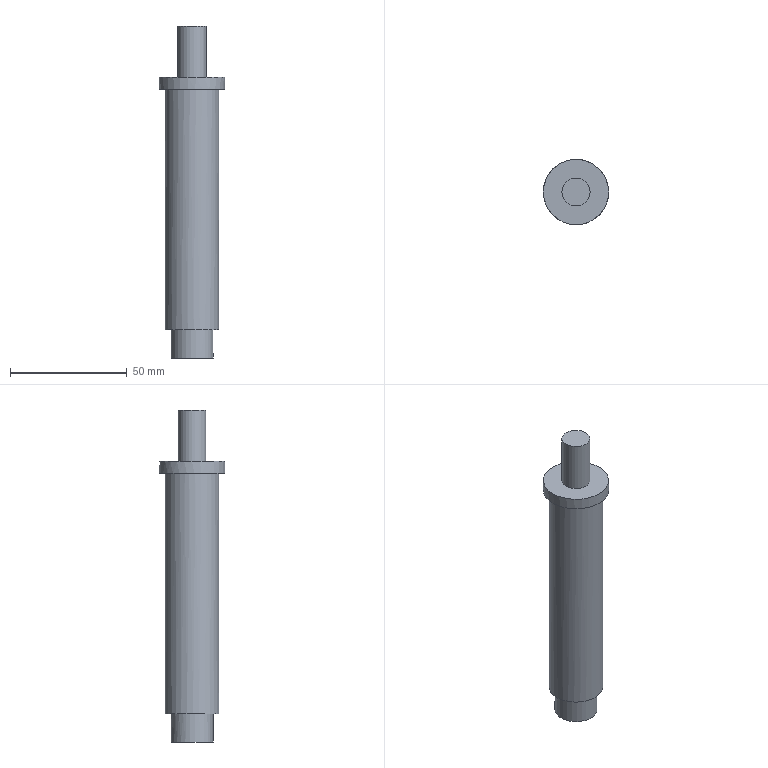Part | NX | features solid 2 | 1 solid | 9 faces | box 28 x 28 x 142 mm | volume 51405 mm3 | cylinder 4 | spline 3 | plane 2 | commonest cylinder face diameters 12 x1 18 x1 23 x1 28 x1
STEP:
#1=CARTESIAN_POINT('',(513.214,-493.679,345.));
#2=VERTEX_POINT('',#1);
#3=CARTESIAN_POINT('',(508.545,-499.324,345.));
#4=CARTESIAN_POINT('',(514.105,-494.076,345.));
#5=CARTESIAN_POINT('',(514.317,-486.444,345.));
#6=CARTESIAN_POINT('',(509.083,-480.902,345.));
#7=CARTESIAN_POINT('',(501.451,-480.677,345.));
#8=CARTESIAN_POINT('',(495.899,-485.922,345.));
#9=CARTESIAN_POINT('',(495.678,-493.543,345.));
#10=CARTESIAN_POINT('',(500.913,-499.098,345.));
#11=CARTESIAN_POINT('',(508.545,-499.324,345.));
#12=CARTESIAN_POINT('',(514.105,-494.076,345.));
#13=CARTESIAN_POINT('',(514.317,-486.444,345.));
#14=B_SPLINE_CURVE_WITH_KNOTS('',3,(#3,#4,#5,#6,#7,#8,#9,#10,#11,#12,#13),.UNSPECIFIED.,.T.,.F.,(1,1,1,1,1,1,1,1,1,1,1,1,1,1,1),(-0.0211,-0.01407,-0.007034,0.,0.007034,0.01407,0.0211,0.02813,0.03517,0.0422,0.04924,0.05627,0.0633,0.07034,0.07737),.UNSPECIFIED.);
#15=EDGE_CURVE('',#2,#2,#14,.T.);
#16=ORIENTED_EDGE('',*,*,#15,.F.);
#17=EDGE_LOOP('',(#16));
#18=FACE_BOUND('',#17,.T.);
#19=CARTESIAN_POINT('',(514.161,-499.158,345.));
#20=CARTESIAN_POINT('',(514.161,-493.06,345.));
#21=CARTESIAN_POINT('',(514.161,-486.962,345.));
#22=CARTESIAN_POINT('',(514.161,-480.864,345.));
#23=CARTESIAN_POINT('',(508.055,-499.158,345.));
#24=CARTESIAN_POINT('',(508.055,-493.06,345.));
#25=CARTESIAN_POINT('',(508.055,-486.962,345.));
#26=CARTESIAN_POINT('',(508.055,-480.864,345.));
#27=CARTESIAN_POINT('',(501.948,-499.158,345.));
#28=CARTESIAN_POINT('',(501.948,-493.06,345.));
#29=CARTESIAN_POINT('',(501.948,-486.962,345.));
#30=CARTESIAN_POINT('',(501.948,-480.864,345.));
#31=CARTESIAN_POINT('',(495.841,-499.158,345.));
#32=CARTESIAN_POINT('',(495.841,-493.06,345.));
#33=CARTESIAN_POINT('',(495.841,-486.962,345.));
#34=CARTESIAN_POINT('',(495.841,-480.864,345.));
#35=B_SPLINE_SURFACE_WITH_KNOTS('',3,3,((#19,#20,#21,#22),(#23,#24,#25,#26),(#27,#28,#29,#30),(#31,#32,#33,#34)),.UNSPECIFIED.,.F.,.F.,.F.,(4,4),(4,4),(0.3104,0.6896),(0.3104,0.6891),.UNSPECIFIED.);
#36=ADVANCED_FACE('',(#18),#35,.T.);
#37=CARTESIAN_POINT('',(496.05,-489.054,357.));
#38=VERTEX_POINT('',#37);
#39=CARTESIAN_POINT('',(498.734,-482.238,357.));
#40=CARTESIAN_POINT('',(495.079,-488.954,357.));
#41=CARTESIAN_POINT('',(497.249,-496.273,357.));
#42=CARTESIAN_POINT('',(503.945,-499.916,357.));
#43=CARTESIAN_POINT('',(511.269,-497.759,357.));
#44=CARTESIAN_POINT('',(514.917,-491.049,357.));
#45=CARTESIAN_POINT('',(512.76,-483.737,357.));
#46=CARTESIAN_POINT('',(506.059,-480.082,357.));
#47=CARTESIAN_POINT('',(498.734,-482.238,357.));
#48=CARTESIAN_POINT('',(495.079,-488.954,357.));
#49=CARTESIAN_POINT('',(497.249,-496.273,357.));
#50=B_SPLINE_CURVE_WITH_KNOTS('',3,(#39,#40,#41,#42,#43,#44,#45,#46,#47,#48,#49),.UNSPECIFIED.,.T.,.F.,(1,1,1,1,1,1,1,1,1,1,1,1,1,1,1),(-0.0211,-0.01407,-0.007034,0.,0.007034,0.01407,0.0211,0.02813,0.03517,0.0422,0.04924,0.05627,0.0633,0.07034,0.07737),.UNSPECIFIED.);
#51=EDGE_CURVE('',#38,#38,#50,.T.);
#52=ORIENTED_EDGE('',*,*,#51,.F.);
#53=EDGE_LOOP('',(#52));
#54=FACE_BOUND('',#53,.T.);
#55=ORIENTED_EDGE('',*,*,#15,.T.);
#56=EDGE_LOOP('',(#55));
#57=FACE_BOUND('',#56,.T.);
#58=CARTESIAN_POINT('',(505.,-490.,405.));
#59=DIRECTION('',(0.,0.,1.));
#60=DIRECTION('',(1.,0.,0.));
#61=AXIS2_PLACEMENT_3D('',#58,#59,#60);
#62=CYLINDRICAL_SURFACE('',#61,9.);
#63=ADVANCED_FACE('',(#54,#57),#62,.T.);
#64=CARTESIAN_POINT('',(493.564,-488.792,460.));
#65=VERTEX_POINT('',#64);
#66=CARTESIAN_POINT('',(496.993,-480.082,460.));
#67=CARTESIAN_POINT('',(492.323,-488.663,460.));
#68=CARTESIAN_POINT('',(495.095,-498.016,460.));
#69=CARTESIAN_POINT('',(503.652,-502.671,460.));
#70=CARTESIAN_POINT('',(513.01,-499.914,460.));
#71=CARTESIAN_POINT('',(517.672,-491.341,460.));
#72=CARTESIAN_POINT('',(514.916,-481.998,460.));
#73=CARTESIAN_POINT('',(506.353,-477.327,460.));
#74=CARTESIAN_POINT('',(496.993,-480.082,460.));
#75=CARTESIAN_POINT('',(492.323,-488.663,460.));
#76=CARTESIAN_POINT('',(495.095,-498.016,460.));
#77=B_SPLINE_CURVE_WITH_KNOTS('',3,(#66,#67,#68,#69,#70,#71,#72,#73,#74,#75,#76),.UNSPECIFIED.,.T.,.F.,(1,1,1,1,1,1,1,1,1,1,1,1,1,1,1),(-0.02696,-0.01798,-0.008988,0.,0.008988,0.01798,0.02696,0.03595,0.04494,0.05393,0.06291,0.0719,0.08089,0.08988,0.09886),.UNSPECIFIED.);
#78=EDGE_CURVE('',#65,#65,#77,.T.);
#79=ORIENTED_EDGE('',*,*,#78,.F.);
#80=EDGE_LOOP('',(#79));
#81=FACE_BOUND('',#80,.T.);
#82=CARTESIAN_POINT('',(516.5,-490.,357.));
#83=VERTEX_POINT('',#82);
#84=CARTESIAN_POINT('',(514.005,-499.022,357.));
#85=CARTESIAN_POINT('',(517.747,-489.998,357.));
#86=CARTESIAN_POINT('',(514.007,-480.987,357.));
#87=CARTESIAN_POINT('',(505.009,-477.258,357.));
#88=CARTESIAN_POINT('',(495.992,-480.982,357.));
#89=CARTESIAN_POINT('',(492.257,-489.998,357.));
#90=CARTESIAN_POINT('',(495.98,-499.,357.));
#91=CARTESIAN_POINT('',(504.986,-502.745,357.));
#92=CARTESIAN_POINT('',(514.005,-499.022,357.));
#93=CARTESIAN_POINT('',(517.747,-489.998,357.));
#94=CARTESIAN_POINT('',(514.007,-480.987,357.));
#95=B_SPLINE_CURVE_WITH_KNOTS('',3,(#84,#85,#86,#87,#88,#89,#90,#91,#92,#93,#94),.UNSPECIFIED.,.T.,.F.,(1,1,1,1,1,1,1,1,1,1,1,1,1,1,1),(-0.02696,-0.01798,-0.008988,0.,0.008988,0.01798,0.02696,0.03595,0.04494,0.05393,0.06291,0.0719,0.08089,0.08988,0.09886),.UNSPECIFIED.);
#96=EDGE_CURVE('',#83,#83,#95,.T.);
#97=ORIENTED_EDGE('',*,*,#96,.T.);
#98=EDGE_LOOP('',(#97));
#99=FACE_BOUND('',#98,.T.);
#100=CARTESIAN_POINT('',(505.,-490.,405.));
#101=DIRECTION('',(0.,0.,1.));
#102=DIRECTION('',(1.,0.,0.));
#103=AXIS2_PLACEMENT_3D('',#100,#101,#102);
#104=CYLINDRICAL_SURFACE('',#103,11.5);
#105=ADVANCED_FACE('',(#81,#99),#104,.T.);
#106=ORIENTED_EDGE('',*,*,#78,.T.);
#107=EDGE_LOOP('',(#106));
#108=FACE_BOUND('',#107,.T.);
#109=CARTESIAN_POINT('',(519.,-490.,460.));
#110=VERTEX_POINT('',#109);
#111=CARTESIAN_POINT('',(515.962,-500.983,460.));
#112=CARTESIAN_POINT('',(520.518,-489.997,460.));
#113=CARTESIAN_POINT('',(515.966,-479.028,460.));
#114=CARTESIAN_POINT('',(505.011,-474.487,460.));
#115=CARTESIAN_POINT('',(494.034,-479.022,460.));
#116=CARTESIAN_POINT('',(489.487,-489.998,460.));
#117=CARTESIAN_POINT('',(494.019,-500.957,460.));
#118=CARTESIAN_POINT('',(504.983,-505.515,460.));
#119=CARTESIAN_POINT('',(515.962,-500.983,460.));
#120=CARTESIAN_POINT('',(520.518,-489.997,460.));
#121=CARTESIAN_POINT('',(515.966,-479.028,460.));
#122=B_SPLINE_CURVE_WITH_KNOTS('',3,(#111,#112,#113,#114,#115,#116,#117,#118,#119,#120,#121),.UNSPECIFIED.,.T.,.F.,(1,1,1,1,1,1,1,1,1,1,1,1,1,1,1),(-0.03282,-0.02188,-0.01094,0.,0.01094,0.02188,0.03282,0.04377,0.05471,0.06565,0.07659,0.08753,0.09847,0.1094,0.1204),.UNSPECIFIED.);
#123=EDGE_CURVE('',#110,#110,#122,.T.);
#124=ORIENTED_EDGE('',*,*,#123,.F.);
#125=EDGE_LOOP('',(#124));
#126=FACE_BOUND('',#125,.T.);
#127=CARTESIAN_POINT('',(519.169,-504.185,460.));
#128=CARTESIAN_POINT('',(519.169,-475.744,460.));
#129=CARTESIAN_POINT('',(490.744,-504.185,460.));
#130=CARTESIAN_POINT('',(490.744,-475.744,460.));
#131=B_SPLINE_SURFACE_WITH_KNOTS('',1,1,((#127,#128),(#129,#130)),.PLANE_SURF.,.F.,.F.,.F.,(2,2),(2,2),(0.2067,0.7951),(0.2064,0.7951),.PIECEWISE_BEZIER_KNOTS.);
#132=ADVANCED_FACE('',(#108,#126),#131,.T.);
#133=CARTESIAN_POINT('',(511.,-490.,487.));
#134=VERTEX_POINT('',#133);
#135=CARTESIAN_POINT('',(505.,-490.,487.));
#136=DIRECTION('',(0.,0.,-1.));
#137=DIRECTION('',(1.,0.,0.));
#138=AXIS2_PLACEMENT_3D('',#135,#136,#137);
#139=CIRCLE('',#138,6.);
#140=EDGE_CURVE('',#134,#134,#139,.T.);
#141=ORIENTED_EDGE('',*,*,#140,.F.);
#142=EDGE_LOOP('',(#141));
#143=FACE_BOUND('',#142,.T.);
#144=CARTESIAN_POINT('',(505.,-484.,487.));
#145=DIRECTION('',(0.,0.,-1.));
#146=DIRECTION('',(-1.,0.,0.));
#147=AXIS2_PLACEMENT_3D('',#144,#145,#146);
#148=PLANE('',#147);
#149=ADVANCED_FACE('',(#143),#148,.F.);
#150=ORIENTED_EDGE('',*,*,#140,.T.);
#151=EDGE_LOOP('',(#150));
#152=FACE_BOUND('',#151,.T.);
#153=CARTESIAN_POINT('',(511.,-490.,465.));
#154=VERTEX_POINT('',#153);
#155=CARTESIAN_POINT('',(505.,-490.,465.));
#156=DIRECTION('',(0.,0.,-1.));
#157=DIRECTION('',(1.,0.,0.));
#158=AXIS2_PLACEMENT_3D('',#155,#156,#157);
#159=CIRCLE('',#158,6.);
#160=EDGE_CURVE('',#154,#154,#159,.T.);
#161=ORIENTED_EDGE('',*,*,#160,.F.);
#162=EDGE_LOOP('',(#161));
#163=FACE_BOUND('',#162,.T.);
#164=CARTESIAN_POINT('',(505.,-490.,385.));
#165=DIRECTION('',(0.,0.,1.));
#166=DIRECTION('',(1.,0.,0.));
#167=AXIS2_PLACEMENT_3D('',#164,#165,#166);
#168=CYLINDRICAL_SURFACE('',#167,6.);
#169=ADVANCED_FACE('',(#152,#163),#168,.T.);
#170=ORIENTED_EDGE('',*,*,#160,.T.);
#171=EDGE_LOOP('',(#170));
#172=FACE_BOUND('',#171,.T.);
#173=CARTESIAN_POINT('',(519.,-490.,465.));
#174=VERTEX_POINT('',#173);
#175=CARTESIAN_POINT('',(505.,-490.,465.));
#176=DIRECTION('',(0.,0.,-1.));
#177=DIRECTION('',(1.,0.,0.));
#178=AXIS2_PLACEMENT_3D('',#175,#176,#177);
#179=CIRCLE('',#178,14.);
#180=EDGE_CURVE('',#174,#174,#179,.T.);
#181=ORIENTED_EDGE('',*,*,#180,.F.);
#182=EDGE_LOOP('',(#181));
#183=FACE_BOUND('',#182,.T.);
#184=CARTESIAN_POINT('',(505.,-476.,465.));
#185=DIRECTION('',(0.,0.,-1.));
#186=DIRECTION('',(-1.,0.,0.));
#187=AXIS2_PLACEMENT_3D('',#184,#185,#186);
#188=PLANE('',#187);
#189=ADVANCED_FACE('',(#172,#183),#188,.F.);
#190=ORIENTED_EDGE('',*,*,#180,.T.);
#191=EDGE_LOOP('',(#190));
#192=FACE_BOUND('',#191,.T.);
#193=ORIENTED_EDGE('',*,*,#123,.T.);
#194=EDGE_LOOP('',(#193));
#195=FACE_BOUND('',#194,.T.);
#196=CARTESIAN_POINT('',(505.,-490.,405.));
#197=DIRECTION('',(0.,0.,1.));
#198=DIRECTION('',(1.,0.,0.));
#199=AXIS2_PLACEMENT_3D('',#196,#197,#198);
#200=CYLINDRICAL_SURFACE('',#199,14.);
#201=ADVANCED_FACE('',(#192,#195),#200,.T.);
#202=ORIENTED_EDGE('',*,*,#51,.T.);
#203=EDGE_LOOP('',(#202));
#204=FACE_BOUND('',#203,.T.);
#205=ORIENTED_EDGE('',*,*,#96,.F.);
#206=EDGE_LOOP('',(#205));
#207=FACE_BOUND('',#206,.T.);
#208=CARTESIAN_POINT('',(516.638,-501.652,357.));
#209=CARTESIAN_POINT('',(516.638,-478.29,357.));
#210=CARTESIAN_POINT('',(493.29,-501.652,357.));
#211=CARTESIAN_POINT('',(493.29,-478.29,357.));
#212=B_SPLINE_SURFACE_WITH_KNOTS('',1,1,((#208,#209),(#210,#211)),.PLANE_SURF.,.F.,.F.,.F.,(2,2),(2,2),(0.2519,0.7496),(0.2517,0.7496),.PIECEWISE_BEZIER_KNOTS.);
#213=ADVANCED_FACE('',(#204,#207),#212,.T.);
#214=CLOSED_SHELL('',(#36,#63,#105,#132,#149,#169,#189,#201,#213));
#215=MANIFOLD_SOLID_BREP('',#214);
#216=(LENGTH_UNIT()NAMED_UNIT(*)SI_UNIT(.MILLI.,.METRE.));
#217=UNCERTAINTY_MEASURE_WITH_UNIT(LENGTH_MEASURE(0.0508),#216,'','');
#218=(NAMED_UNIT(*)PLANE_ANGLE_UNIT()SI_UNIT($,.RADIAN.));
#219=(NAMED_UNIT(*)SI_UNIT($,.STERADIAN.)SOLID_ANGLE_UNIT());
#220=(GEOMETRIC_REPRESENTATION_CONTEXT(3)GLOBAL_UNCERTAINTY_ASSIGNED_CONTEXT((#217))GLOBAL_UNIT_ASSIGNED_CONTEXT((#216,#218,#219))REPRESENTATION_CONTEXT('',''));
#221=ADVANCED_BREP_SHAPE_REPRESENTATION('',(#215),#220);